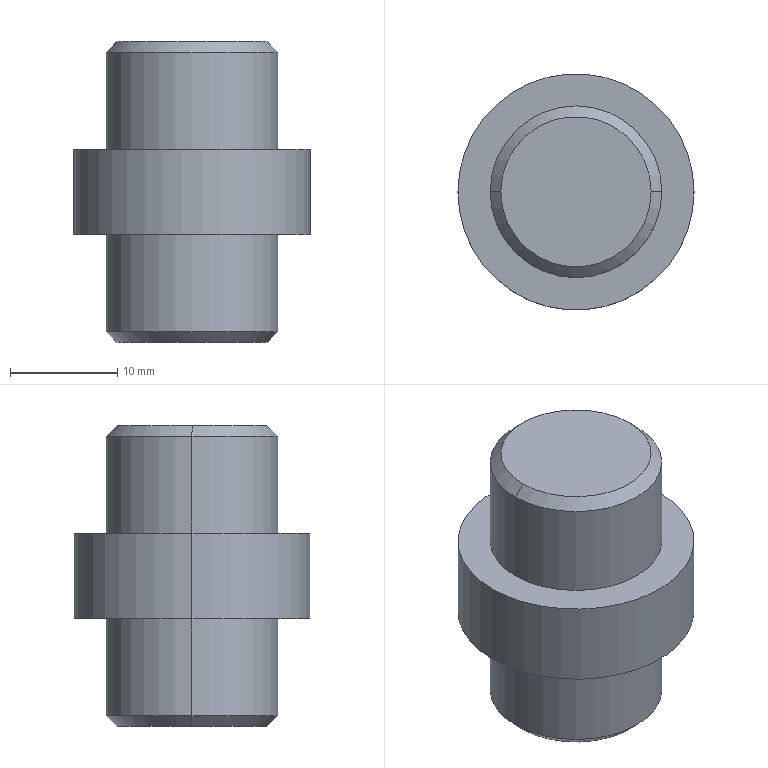Part | SolidWorks | features ICE 2, Chamfer 1, Extrusion 1 | 1 solid | 14 faces | box 22 x 22 x 28 mm | volume 7014 mm3 | cylinder 6 | cone 4 | plane 4 | commonest cylinder face diameters 16 x4 22 x2
STEP:
#1=CARTESIAN_POINT('',(-7.,0.,-10.));
#2=VERTEX_POINT('',#1);
#3=CARTESIAN_POINT('',(7.,0.,-10.));
#4=VERTEX_POINT('',#3);
#5=CARTESIAN_POINT('',(0.,0.,-10.));
#6=DIRECTION('',(0.,0.,-1.));
#7=DIRECTION('',(-1.,0.,0.));
#8=AXIS2_PLACEMENT_3D('',#5,#6,#7);
#9=CIRCLE('',#8,7.);
#10=EDGE_CURVE('',#2,#4,#9,.T.);
#11=ORIENTED_EDGE('',*,*,#10,.F.);
#12=CARTESIAN_POINT('',(-8.,0.,-9.));
#13=VERTEX_POINT('',#12);
#14=CARTESIAN_POINT('',(-7.,0.,-10.));
#15=DIRECTION('',(-0.7071,0.,0.7071));
#16=VECTOR('',#15,1000.);
#17=LINE('',#14,#16);
#18=EDGE_CURVE('',#2,#13,#17,.T.);
#19=ORIENTED_EDGE('',*,*,#18,.T.);
#20=CARTESIAN_POINT('',(8.,0.,-9.));
#21=VERTEX_POINT('',#20);
#22=CARTESIAN_POINT('',(0.,0.,-9.));
#23=DIRECTION('',(0.,0.,1.));
#24=DIRECTION('',(-1.,0.,0.));
#25=AXIS2_PLACEMENT_3D('',#22,#23,#24);
#26=CIRCLE('',#25,8.);
#27=EDGE_CURVE('',#21,#13,#26,.T.);
#28=ORIENTED_EDGE('',*,*,#27,.F.);
#29=CARTESIAN_POINT('',(7.,0.,-10.));
#30=DIRECTION('',(0.7071,0.,0.7071));
#31=VECTOR('',#30,1000.);
#32=LINE('',#29,#31);
#33=EDGE_CURVE('',#4,#21,#32,.T.);
#34=ORIENTED_EDGE('',*,*,#33,.F.);
#35=EDGE_LOOP('',(#11,#19,#28,#34));
#36=FACE_OUTER_BOUND('',#35,.T.);
#37=CARTESIAN_POINT('',(0.,0.,-10.));
#38=DIRECTION('',(0.,0.,1.));
#39=DIRECTION('',(1.,0.,0.));
#40=AXIS2_PLACEMENT_3D('',#37,#38,#39);
#41=CONICAL_SURFACE('',#40,7.,0.7854);
#42=ADVANCED_FACE('',(#36),#41,.T.);
#43=CARTESIAN_POINT('',(7.,0.,18.));
#44=VERTEX_POINT('',#43);
#45=CARTESIAN_POINT('',(-7.,0.,18.));
#46=VERTEX_POINT('',#45);
#47=CARTESIAN_POINT('',(0.,0.,18.));
#48=DIRECTION('',(0.,0.,1.));
#49=DIRECTION('',(1.,0.,0.));
#50=AXIS2_PLACEMENT_3D('',#47,#48,#49);
#51=CIRCLE('',#50,7.);
#52=EDGE_CURVE('',#44,#46,#51,.T.);
#53=ORIENTED_EDGE('',*,*,#52,.F.);
#54=CARTESIAN_POINT('',(8.,0.,17.));
#55=VERTEX_POINT('',#54);
#56=CARTESIAN_POINT('',(7.,0.,18.));
#57=DIRECTION('',(0.7071,0.,-0.7071));
#58=VECTOR('',#57,1000.);
#59=LINE('',#56,#58);
#60=EDGE_CURVE('',#44,#55,#59,.T.);
#61=ORIENTED_EDGE('',*,*,#60,.T.);
#62=CARTESIAN_POINT('',(-8.,0.,17.));
#63=VERTEX_POINT('',#62);
#64=CARTESIAN_POINT('',(0.,0.,17.));
#65=DIRECTION('',(0.,0.,-1.));
#66=DIRECTION('',(1.,0.,0.));
#67=AXIS2_PLACEMENT_3D('',#64,#65,#66);
#68=CIRCLE('',#67,8.);
#69=EDGE_CURVE('',#63,#55,#68,.T.);
#70=ORIENTED_EDGE('',*,*,#69,.F.);
#71=CARTESIAN_POINT('',(-7.,0.,18.));
#72=DIRECTION('',(-0.7071,0.,-0.7071));
#73=VECTOR('',#72,1000.);
#74=LINE('',#71,#73);
#75=EDGE_CURVE('',#46,#63,#74,.T.);
#76=ORIENTED_EDGE('',*,*,#75,.F.);
#77=EDGE_LOOP('',(#53,#61,#70,#76));
#78=FACE_OUTER_BOUND('',#77,.T.);
#79=CARTESIAN_POINT('',(0.,0.,18.));
#80=DIRECTION('',(0.,0.,-1.));
#81=DIRECTION('',(-1.,0.,0.));
#82=AXIS2_PLACEMENT_3D('',#79,#80,#81);
#83=CONICAL_SURFACE('',#82,7.,0.7854);
#84=ADVANCED_FACE('',(#78),#83,.T.);
#85=ORIENTED_EDGE('',*,*,#27,.T.);
#86=CARTESIAN_POINT('',(-8.,0.,0.));
#87=VERTEX_POINT('',#86);
#88=CARTESIAN_POINT('',(-8.,0.,-10.));
#89=DIRECTION('',(0.,0.,1.));
#90=VECTOR('',#89,1000.);
#91=LINE('',#88,#90);
#92=EDGE_CURVE('',#13,#87,#91,.T.);
#93=ORIENTED_EDGE('',*,*,#92,.T.);
#94=CARTESIAN_POINT('',(8.,0.,0.));
#95=VERTEX_POINT('',#94);
#96=CARTESIAN_POINT('',(0.,0.,0.));
#97=DIRECTION('',(0.,0.,-1.));
#98=DIRECTION('',(-1.,0.,0.));
#99=AXIS2_PLACEMENT_3D('',#96,#97,#98);
#100=CIRCLE('',#99,8.);
#101=EDGE_CURVE('',#87,#95,#100,.T.);
#102=ORIENTED_EDGE('',*,*,#101,.T.);
#103=CARTESIAN_POINT('',(8.,0.,-10.));
#104=DIRECTION('',(0.,0.,1.));
#105=VECTOR('',#104,1000.);
#106=LINE('',#103,#105);
#107=EDGE_CURVE('',#21,#95,#106,.T.);
#108=ORIENTED_EDGE('',*,*,#107,.F.);
#109=EDGE_LOOP('',(#85,#93,#102,#108));
#110=FACE_OUTER_BOUND('',#109,.T.);
#111=CARTESIAN_POINT('',(0.,0.,-10.));
#112=DIRECTION('',(0.,0.,1.));
#113=DIRECTION('',(1.,0.,0.));
#114=AXIS2_PLACEMENT_3D('',#111,#112,#113);
#115=CYLINDRICAL_SURFACE('',#114,8.);
#116=ADVANCED_FACE('',(#110),#115,.T.);
#117=ORIENTED_EDGE('',*,*,#69,.T.);
#118=CARTESIAN_POINT('',(8.,0.,8.));
#119=VERTEX_POINT('',#118);
#120=CARTESIAN_POINT('',(8.,0.,18.));
#121=DIRECTION('',(0.,0.,-1.));
#122=VECTOR('',#121,1000.);
#123=LINE('',#120,#122);
#124=EDGE_CURVE('',#55,#119,#123,.T.);
#125=ORIENTED_EDGE('',*,*,#124,.T.);
#126=CARTESIAN_POINT('',(-8.,0.,8.));
#127=VERTEX_POINT('',#126);
#128=CARTESIAN_POINT('',(0.,0.,8.));
#129=DIRECTION('',(0.,0.,1.));
#130=DIRECTION('',(1.,0.,0.));
#131=AXIS2_PLACEMENT_3D('',#128,#129,#130);
#132=CIRCLE('',#131,8.);
#133=EDGE_CURVE('',#119,#127,#132,.T.);
#134=ORIENTED_EDGE('',*,*,#133,.T.);
#135=CARTESIAN_POINT('',(-8.,0.,18.));
#136=DIRECTION('',(0.,0.,-1.));
#137=VECTOR('',#136,1000.);
#138=LINE('',#135,#137);
#139=EDGE_CURVE('',#63,#127,#138,.T.);
#140=ORIENTED_EDGE('',*,*,#139,.F.);
#141=EDGE_LOOP('',(#117,#125,#134,#140));
#142=FACE_OUTER_BOUND('',#141,.T.);
#143=CARTESIAN_POINT('',(0.,0.,18.));
#144=DIRECTION('',(0.,0.,-1.));
#145=DIRECTION('',(-1.,0.,0.));
#146=AXIS2_PLACEMENT_3D('',#143,#144,#145);
#147=CYLINDRICAL_SURFACE('',#146,8.);
#148=ADVANCED_FACE('',(#142),#147,.T.);
#149=CARTESIAN_POINT('',(11.,0.,8.));
#150=VERTEX_POINT('',#149);
#151=CARTESIAN_POINT('',(-11.,0.,8.));
#152=VERTEX_POINT('',#151);
#153=CARTESIAN_POINT('',(0.,0.,8.));
#154=DIRECTION('',(0.,0.,1.));
#155=DIRECTION('',(1.,0.,0.));
#156=AXIS2_PLACEMENT_3D('',#153,#154,#155);
#157=CIRCLE('',#156,11.);
#158=EDGE_CURVE('',#150,#152,#157,.T.);
#159=ORIENTED_EDGE('',*,*,#158,.F.);
#160=CARTESIAN_POINT('',(11.,0.,0.));
#161=VERTEX_POINT('',#160);
#162=CARTESIAN_POINT('',(11.,0.,8.));
#163=DIRECTION('',(0.,0.,-1.));
#164=VECTOR('',#163,1000.);
#165=LINE('',#162,#164);
#166=EDGE_CURVE('',#150,#161,#165,.T.);
#167=ORIENTED_EDGE('',*,*,#166,.T.);
#168=CARTESIAN_POINT('',(-11.,0.,0.));
#169=VERTEX_POINT('',#168);
#170=CARTESIAN_POINT('',(0.,0.,0.));
#171=DIRECTION('',(0.,0.,1.));
#172=DIRECTION('',(1.,0.,0.));
#173=AXIS2_PLACEMENT_3D('',#170,#171,#172);
#174=CIRCLE('',#173,11.);
#175=EDGE_CURVE('',#161,#169,#174,.T.);
#176=ORIENTED_EDGE('',*,*,#175,.T.);
#177=CARTESIAN_POINT('',(-11.,0.,8.));
#178=DIRECTION('',(0.,0.,-1.));
#179=VECTOR('',#178,1000.);
#180=LINE('',#177,#179);
#181=EDGE_CURVE('',#152,#169,#180,.T.);
#182=ORIENTED_EDGE('',*,*,#181,.F.);
#183=EDGE_LOOP('',(#159,#167,#176,#182));
#184=FACE_OUTER_BOUND('',#183,.T.);
#185=CARTESIAN_POINT('',(0.,0.,8.));
#186=DIRECTION('',(0.,0.,-1.));
#187=DIRECTION('',(-1.,0.,0.));
#188=AXIS2_PLACEMENT_3D('',#185,#186,#187);
#189=CYLINDRICAL_SURFACE('',#188,11.);
#190=ADVANCED_FACE('',(#184),#189,.T.);
#191=ORIENTED_EDGE('',*,*,#166,.F.);
#192=CARTESIAN_POINT('',(0.,0.,8.));
#193=DIRECTION('',(0.,0.,1.));
#194=DIRECTION('',(1.,0.,0.));
#195=AXIS2_PLACEMENT_3D('',#192,#193,#194);
#196=CIRCLE('',#195,11.);
#197=EDGE_CURVE('',#152,#150,#196,.T.);
#198=ORIENTED_EDGE('',*,*,#197,.F.);
#199=ORIENTED_EDGE('',*,*,#181,.T.);
#200=CARTESIAN_POINT('',(0.,0.,0.));
#201=DIRECTION('',(0.,0.,1.));
#202=DIRECTION('',(1.,0.,0.));
#203=AXIS2_PLACEMENT_3D('',#200,#201,#202);
#204=CIRCLE('',#203,11.);
#205=EDGE_CURVE('',#169,#161,#204,.T.);
#206=ORIENTED_EDGE('',*,*,#205,.T.);
#207=EDGE_LOOP('',(#191,#198,#199,#206));
#208=FACE_OUTER_BOUND('',#207,.T.);
#209=CARTESIAN_POINT('',(0.,0.,8.));
#210=DIRECTION('',(0.,0.,-1.));
#211=DIRECTION('',(-1.,0.,0.));
#212=AXIS2_PLACEMENT_3D('',#209,#210,#211);
#213=CYLINDRICAL_SURFACE('',#212,11.);
#214=ADVANCED_FACE('',(#208),#213,.T.);
#215=CARTESIAN_POINT('',(0.,0.,8.));
#216=DIRECTION('',(0.,0.,1.));
#217=DIRECTION('',(1.,0.,0.));
#218=AXIS2_PLACEMENT_3D('',#215,#216,#217);
#219=CIRCLE('',#218,8.);
#220=EDGE_CURVE('',#127,#119,#219,.T.);
#221=ORIENTED_EDGE('',*,*,#220,.F.);
#222=ORIENTED_EDGE('',*,*,#133,.F.);
#223=EDGE_LOOP('',(#221,#222));
#224=FACE_BOUND('',#223,.T.);
#225=ORIENTED_EDGE('',*,*,#197,.T.);
#226=ORIENTED_EDGE('',*,*,#158,.T.);
#227=EDGE_LOOP('',(#225,#226));
#228=FACE_OUTER_BOUND('',#227,.T.);
#229=CARTESIAN_POINT('',(0.,0.,8.));
#230=DIRECTION('',(0.,0.,1.));
#231=DIRECTION('',(1.,0.,0.));
#232=AXIS2_PLACEMENT_3D('',#229,#230,#231);
#233=PLANE('',#232);
#234=ADVANCED_FACE('',(#224,#228),#233,.T.);
#235=CARTESIAN_POINT('',(0.,0.,0.));
#236=DIRECTION('',(0.,0.,-1.));
#237=DIRECTION('',(-1.,0.,0.));
#238=AXIS2_PLACEMENT_3D('',#235,#236,#237);
#239=CIRCLE('',#238,8.);
#240=EDGE_CURVE('',#95,#87,#239,.T.);
#241=ORIENTED_EDGE('',*,*,#240,.F.);
#242=ORIENTED_EDGE('',*,*,#101,.F.);
#243=EDGE_LOOP('',(#241,#242));
#244=FACE_BOUND('',#243,.T.);
#245=ORIENTED_EDGE('',*,*,#205,.F.);
#246=ORIENTED_EDGE('',*,*,#175,.F.);
#247=EDGE_LOOP('',(#245,#246));
#248=FACE_OUTER_BOUND('',#247,.T.);
#249=CARTESIAN_POINT('',(0.,0.,0.));
#250=DIRECTION('',(0.,0.,1.));
#251=DIRECTION('',(1.,0.,0.));
#252=AXIS2_PLACEMENT_3D('',#249,#250,#251);
#253=PLANE('',#252);
#254=ADVANCED_FACE('',(#244,#248),#253,.F.);
#255=ORIENTED_EDGE('',*,*,#124,.F.);
#256=CARTESIAN_POINT('',(0.,0.,17.));
#257=DIRECTION('',(0.,0.,-1.));
#258=DIRECTION('',(1.,0.,0.));
#259=AXIS2_PLACEMENT_3D('',#256,#257,#258);
#260=CIRCLE('',#259,8.);
#261=EDGE_CURVE('',#55,#63,#260,.T.);
#262=ORIENTED_EDGE('',*,*,#261,.T.);
#263=ORIENTED_EDGE('',*,*,#139,.T.);
#264=ORIENTED_EDGE('',*,*,#220,.T.);
#265=EDGE_LOOP('',(#255,#262,#263,#264));
#266=FACE_OUTER_BOUND('',#265,.T.);
#267=CARTESIAN_POINT('',(0.,0.,18.));
#268=DIRECTION('',(0.,0.,-1.));
#269=DIRECTION('',(-1.,0.,0.));
#270=AXIS2_PLACEMENT_3D('',#267,#268,#269);
#271=CYLINDRICAL_SURFACE('',#270,8.);
#272=ADVANCED_FACE('',(#266),#271,.T.);
#273=CARTESIAN_POINT('',(0.,0.,18.));
#274=DIRECTION('',(0.,0.,1.));
#275=DIRECTION('',(1.,0.,0.));
#276=AXIS2_PLACEMENT_3D('',#273,#274,#275);
#277=CIRCLE('',#276,7.);
#278=EDGE_CURVE('',#46,#44,#277,.T.);
#279=ORIENTED_EDGE('',*,*,#278,.T.);
#280=ORIENTED_EDGE('',*,*,#52,.T.);
#281=EDGE_LOOP('',(#279,#280));
#282=FACE_OUTER_BOUND('',#281,.T.);
#283=CARTESIAN_POINT('',(0.,0.,18.));
#284=DIRECTION('',(0.,0.,1.));
#285=DIRECTION('',(1.,0.,0.));
#286=AXIS2_PLACEMENT_3D('',#283,#284,#285);
#287=PLANE('',#286);
#288=ADVANCED_FACE('',(#282),#287,.T.);
#289=ORIENTED_EDGE('',*,*,#92,.F.);
#290=CARTESIAN_POINT('',(0.,0.,-9.));
#291=DIRECTION('',(0.,0.,1.));
#292=DIRECTION('',(-1.,0.,0.));
#293=AXIS2_PLACEMENT_3D('',#290,#291,#292);
#294=CIRCLE('',#293,8.);
#295=EDGE_CURVE('',#13,#21,#294,.T.);
#296=ORIENTED_EDGE('',*,*,#295,.T.);
#297=ORIENTED_EDGE('',*,*,#107,.T.);
#298=ORIENTED_EDGE('',*,*,#240,.T.);
#299=EDGE_LOOP('',(#289,#296,#297,#298));
#300=FACE_OUTER_BOUND('',#299,.T.);
#301=CARTESIAN_POINT('',(0.,0.,-10.));
#302=DIRECTION('',(0.,0.,1.));
#303=DIRECTION('',(1.,0.,0.));
#304=AXIS2_PLACEMENT_3D('',#301,#302,#303);
#305=CYLINDRICAL_SURFACE('',#304,8.);
#306=ADVANCED_FACE('',(#300),#305,.T.);
#307=CARTESIAN_POINT('',(0.,0.,-10.));
#308=DIRECTION('',(0.,0.,-1.));
#309=DIRECTION('',(-1.,0.,0.));
#310=AXIS2_PLACEMENT_3D('',#307,#308,#309);
#311=CIRCLE('',#310,7.);
#312=EDGE_CURVE('',#4,#2,#311,.T.);
#313=ORIENTED_EDGE('',*,*,#312,.T.);
#314=ORIENTED_EDGE('',*,*,#10,.T.);
#315=EDGE_LOOP('',(#313,#314));
#316=FACE_OUTER_BOUND('',#315,.T.);
#317=CARTESIAN_POINT('',(0.,0.,-10.));
#318=DIRECTION('',(0.,0.,-1.));
#319=DIRECTION('',(-1.,0.,0.));
#320=AXIS2_PLACEMENT_3D('',#317,#318,#319);
#321=PLANE('',#320);
#322=ADVANCED_FACE('',(#316),#321,.T.);
#323=ORIENTED_EDGE('',*,*,#60,.F.);
#324=ORIENTED_EDGE('',*,*,#278,.F.);
#325=ORIENTED_EDGE('',*,*,#75,.T.);
#326=ORIENTED_EDGE('',*,*,#261,.F.);
#327=EDGE_LOOP('',(#323,#324,#325,#326));
#328=FACE_OUTER_BOUND('',#327,.T.);
#329=CARTESIAN_POINT('',(0.,0.,18.));
#330=DIRECTION('',(0.,0.,-1.));
#331=DIRECTION('',(-1.,0.,0.));
#332=AXIS2_PLACEMENT_3D('',#329,#330,#331);
#333=CONICAL_SURFACE('',#332,7.,0.7854);
#334=ADVANCED_FACE('',(#328),#333,.T.);
#335=ORIENTED_EDGE('',*,*,#18,.F.);
#336=ORIENTED_EDGE('',*,*,#312,.F.);
#337=ORIENTED_EDGE('',*,*,#33,.T.);
#338=ORIENTED_EDGE('',*,*,#295,.F.);
#339=EDGE_LOOP('',(#335,#336,#337,#338));
#340=FACE_OUTER_BOUND('',#339,.T.);
#341=CARTESIAN_POINT('',(0.,0.,-10.));
#342=DIRECTION('',(0.,0.,1.));
#343=DIRECTION('',(1.,0.,0.));
#344=AXIS2_PLACEMENT_3D('',#341,#342,#343);
#345=CONICAL_SURFACE('',#344,7.,0.7854);
#346=ADVANCED_FACE('',(#340),#345,.T.);
#347=CLOSED_SHELL('',(#42,#84,#116,#148,#190,#214,#234,#254,#272,#288,#306,#322,#334,#346));
#348=MANIFOLD_SOLID_BREP('',#347);
#349=CARTESIAN_POINT('',(0.,0.,0.));
#350=DIRECTION('',(0.,0.,1.));
#351=DIRECTION('',(1.,0.,0.));
#352=AXIS2_PLACEMENT_3D('',#349,#350,#351);
#353=(LENGTH_UNIT()NAMED_UNIT(*)SI_UNIT(.MILLI.,.METRE.));
#354=UNCERTAINTY_MEASURE_WITH_UNIT(LENGTH_MEASURE(0.00001),#353,'','');
#355=(NAMED_UNIT(*)PLANE_ANGLE_UNIT()SI_UNIT($,.RADIAN.));
#356=(NAMED_UNIT(*)SI_UNIT($,.STERADIAN.)SOLID_ANGLE_UNIT());
#357=(GEOMETRIC_REPRESENTATION_CONTEXT(3)GLOBAL_UNCERTAINTY_ASSIGNED_CONTEXT((#354))GLOBAL_UNIT_ASSIGNED_CONTEXT((#353,#355,#356))REPRESENTATION_CONTEXT('',''));
#358=ADVANCED_BREP_SHAPE_REPRESENTATION('',(#348,#352),#357);